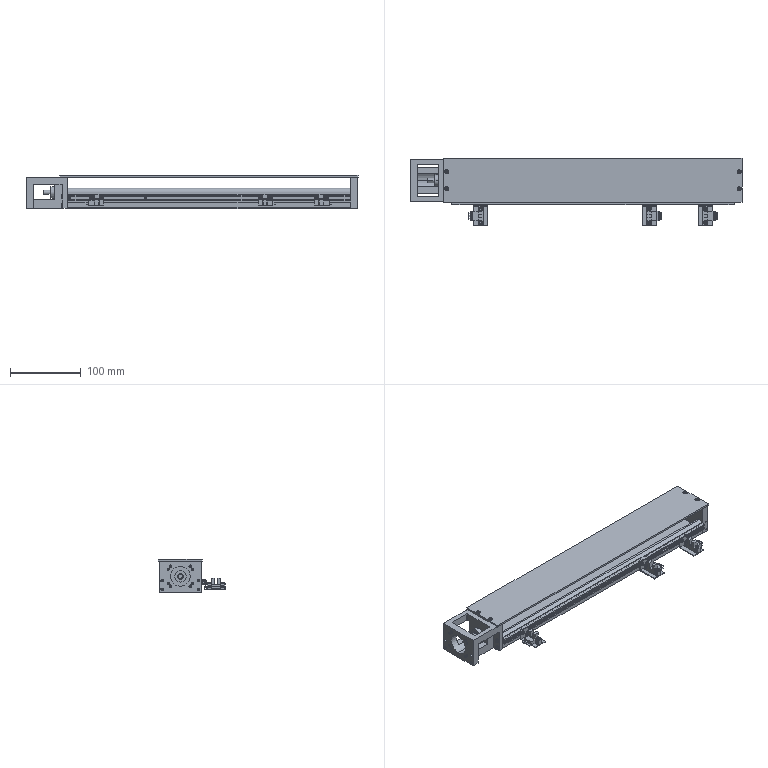Part | STEP file | PRODUCT_ID_1-C-F0-400 | 1 solid | 971 faces | box 470.02 x 94.86 x 47 mm | volume 498801 mm3 | plane 533 | cylinder 260 | cone 138 | spline 40 | commonest cylinder face diameters 5.5 x56 3.19 x24 1.2 x20 2 x20 3.21 x18 2.113 x16